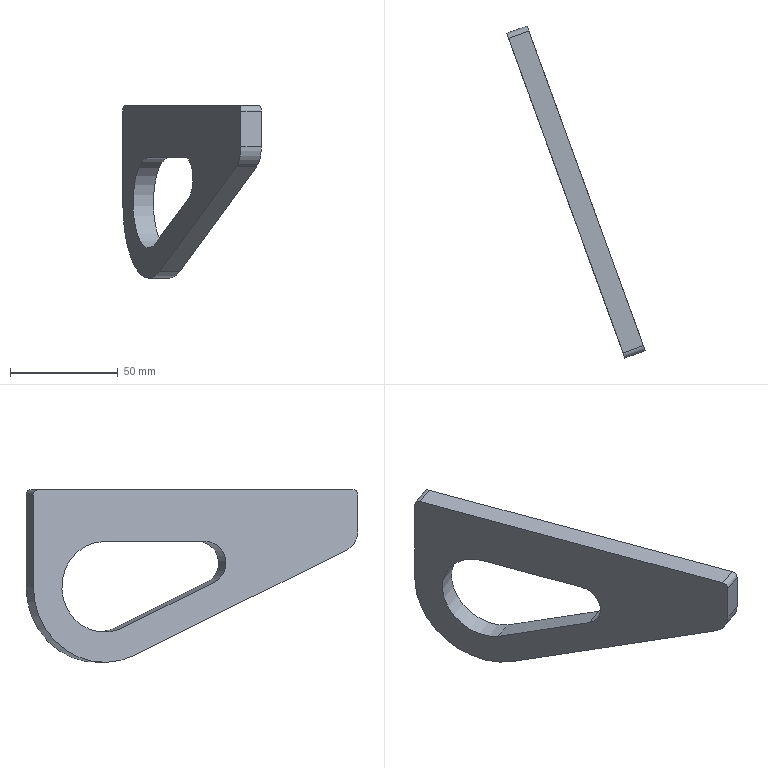Part | STEP file | Input 13 | 1 solid | 14 faces | box 64.12 x 153.771 x 80 mm | volume 68539 mm3 | plane 8 | cylinder 6 | commonest cylinder face diameters 5 x2 19.776 x1 20 x1 42 x1 70 x1
STEP:
#1=CARTESIAN_POINT('',(0.,0.,0.));
#2=DIRECTION('',(0.,0.,1.));
#3=DIRECTION('',(1.,0.,0.));
#4=AXIS2_PLACEMENT_3D('',#1,#2,#3);
#5=CARTESIAN_POINT('',(-156.648,51.655,-248.022));
#6=VERTEX_POINT('',#5);
#7=CARTESIAN_POINT('',(-154.674,46.229,-238.959));
#8=VERTEX_POINT('',#7);
#9=CARTESIAN_POINT('',(-158.094,55.626,-238.959));
#10=DIRECTION('',(-0.9397,-0.342,0.));
#11=DIRECTION('',(0.,0.,-1.));
#12=AXIS2_PLACEMENT_3D('',#9,#10,#11);
#13=CIRCLE('',#12,10.);
#14=CARTESIAN_POINT('',(-148.697,59.046,-238.959));
#15=DIRECTION('',(-0.9397,-0.342,0.));
#16=DIRECTION('',(0.,0.,1.));
#17=AXIS2_PLACEMENT_3D('',#14,#15,#16);
#18=CYLINDRICAL_SURFACE('',#17,10.);
#19=CARTESIAN_POINT('',(3.142,10.));
#20=DIRECTION('',(1.,0.));
#21=VECTOR('',#20,1.);
#22=LINE('',#19,#21);
#23=(GEOMETRIC_REPRESENTATION_CONTEXT(2)PARAMETRIC_REPRESENTATION_CONTEXT()REPRESENTATION_CONTEXT('',''));
#24=DEFINITIONAL_REPRESENTATION('',(#22),#23);
#25=PCURVE('',#18,#24);
#26=CARTESIAN_POINT('',(-158.094,55.626,-238.959));
#27=DIRECTION('',(0.9397,0.342,0.));
#28=DIRECTION('',(0.,0.,-1.));
#29=AXIS2_PLACEMENT_3D('',#26,#27,#28);
#30=PLANE('',#29);
#31=CARTESIAN_POINT('',(10.,0.));
#32=CARTESIAN_POINT('',(10.,-17.321));
#33=CARTESIAN_POINT('',(-5.,-8.66));
#34=CARTESIAN_POINT('',(-20.,0.));
#35=CARTESIAN_POINT('',(-5.,8.66));
#36=CARTESIAN_POINT('',(10.,17.321));
#37=CARTESIAN_POINT('',(10.,0.));
#38=(BOUNDED_CURVE()B_SPLINE_CURVE(2,(#31,#32,#33,#34,#35,#36,#37),.UNSPECIFIED.,.T.,.F.)B_SPLINE_CURVE_WITH_KNOTS((1,2,2,2,2,1),(-2.094,0.,2.094,4.189,6.283,8.378),.UNSPECIFIED.)CURVE()GEOMETRIC_REPRESENTATION_ITEM()RATIONAL_B_SPLINE_CURVE((1.,0.5,1.,0.5,1.,0.5,1.))REPRESENTATION_ITEM(''));
#39=(GEOMETRIC_REPRESENTATION_CONTEXT(2)PARAMETRIC_REPRESENTATION_CONTEXT()REPRESENTATION_CONTEXT('',''));
#40=DEFINITIONAL_REPRESENTATION('',(#38),#39);
#41=PCURVE('',#30,#40);
#42=SURFACE_CURVE('',#13,(#25,#41),.PCURVE_S1.);
#43=EDGE_CURVE('',#6,#8,#42,.T.);
#44=ORIENTED_EDGE('',*,*,#43,.F.);
#45=CARTESIAN_POINT('',(-147.252,55.075,-248.022));
#46=VERTEX_POINT('',#45);
#47=CARTESIAN_POINT('',(-147.252,55.075,-248.022));
#48=DIRECTION('',(-0.9397,-0.342,0.));
#49=VECTOR('',#48,1.);
#50=LINE('',#47,#49);
#51=CARTESIAN_POINT('',(3.578,0.));
#52=DIRECTION('',(0.,1.));
#53=VECTOR('',#52,1.);
#54=LINE('',#51,#53);
#55=(GEOMETRIC_REPRESENTATION_CONTEXT(2)PARAMETRIC_REPRESENTATION_CONTEXT()REPRESENTATION_CONTEXT('',''));
#56=DEFINITIONAL_REPRESENTATION('',(#54),#55);
#57=PCURVE('',#18,#56);
#58=CARTESIAN_POINT('',(-147.252,55.075,-248.022));
#59=DIRECTION('',(0.1445,-0.3971,-0.9063));
#60=DIRECTION('',(0.31,-0.8517,0.4226));
#61=AXIS2_PLACEMENT_3D('',#58,#59,#60);
#62=PLANE('',#61);
#63=CARTESIAN_POINT('',(0.,0.));
#64=DIRECTION('',(0.,1.));
#65=VECTOR('',#64,1.);
#66=LINE('',#63,#65);
#67=(GEOMETRIC_REPRESENTATION_CONTEXT(2)PARAMETRIC_REPRESENTATION_CONTEXT()REPRESENTATION_CONTEXT('',''));
#68=DEFINITIONAL_REPRESENTATION('',(#66),#67);
#69=PCURVE('',#62,#68);
#70=SURFACE_CURVE('',#50,(#57,#69),.PCURVE_S1.);
#71=EDGE_CURVE('',#46,#6,#70,.T.);
#72=ORIENTED_EDGE('',*,*,#71,.F.);
#73=CARTESIAN_POINT('',(-145.277,49.649,-238.959));
#74=VERTEX_POINT('',#73);
#75=CARTESIAN_POINT('',(-148.697,59.046,-238.959));
#76=DIRECTION('',(-0.9397,-0.342,0.));
#77=DIRECTION('',(0.,0.,-1.));
#78=AXIS2_PLACEMENT_3D('',#75,#76,#77);
#79=CIRCLE('',#78,10.);
#80=CARTESIAN_POINT('',(3.142,0.));
#81=DIRECTION('',(1.,0.));
#82=VECTOR('',#81,1.);
#83=LINE('',#80,#82);
#84=(GEOMETRIC_REPRESENTATION_CONTEXT(2)PARAMETRIC_REPRESENTATION_CONTEXT()REPRESENTATION_CONTEXT('',''));
#85=DEFINITIONAL_REPRESENTATION('',(#83),#84);
#86=PCURVE('',#18,#85);
#87=CARTESIAN_POINT('',(-148.697,59.046,-238.959));
#88=DIRECTION('',(0.9397,0.342,0.));
#89=DIRECTION('',(0.,0.,-1.));
#90=AXIS2_PLACEMENT_3D('',#87,#88,#89);
#91=PLANE('',#90);
#92=CARTESIAN_POINT('',(10.,0.));
#93=CARTESIAN_POINT('',(10.,-17.321));
#94=CARTESIAN_POINT('',(-5.,-8.66));
#95=CARTESIAN_POINT('',(-20.,0.));
#96=CARTESIAN_POINT('',(-5.,8.66));
#97=CARTESIAN_POINT('',(10.,17.321));
#98=CARTESIAN_POINT('',(10.,0.));
#99=(BOUNDED_CURVE()B_SPLINE_CURVE(2,(#92,#93,#94,#95,#96,#97,#98),.UNSPECIFIED.,.T.,.F.)B_SPLINE_CURVE_WITH_KNOTS((1,2,2,2,2,1),(-2.094,0.,2.094,4.189,6.283,8.378),.UNSPECIFIED.)CURVE()GEOMETRIC_REPRESENTATION_ITEM()RATIONAL_B_SPLINE_CURVE((1.,0.5,1.,0.5,1.,0.5,1.))REPRESENTATION_ITEM(''));
#100=(GEOMETRIC_REPRESENTATION_CONTEXT(2)PARAMETRIC_REPRESENTATION_CONTEXT()REPRESENTATION_CONTEXT('',''));
#101=DEFINITIONAL_REPRESENTATION('',(#99),#100);
#102=PCURVE('',#91,#101);
#103=SURFACE_CURVE('',#79,(#86,#102),.PCURVE_S1.);
#104=EDGE_CURVE('',#46,#74,#103,.T.);
#105=ORIENTED_EDGE('',*,*,#104,.T.);
#106=CARTESIAN_POINT('',(-145.277,49.649,-238.959));
#107=DIRECTION('',(-0.9397,-0.342,0.));
#108=VECTOR('',#107,1.);
#109=LINE('',#106,#108);
#110=CARTESIAN_POINT('',(4.712,0.));
#111=DIRECTION('',(0.,1.));
#112=VECTOR('',#111,1.);
#113=LINE('',#110,#112);
#114=(GEOMETRIC_REPRESENTATION_CONTEXT(2)PARAMETRIC_REPRESENTATION_CONTEXT()REPRESENTATION_CONTEXT('',''));
#115=DEFINITIONAL_REPRESENTATION('',(#113),#114);
#116=PCURVE('',#18,#115);
#117=CARTESIAN_POINT('',(-145.277,49.649,-222.5));
#118=DIRECTION('',(0.342,-0.9397,0.));
#119=DIRECTION('',(0.9397,0.342,0.));
#120=AXIS2_PLACEMENT_3D('',#117,#118,#119);
#121=PLANE('',#120);
#122=CARTESIAN_POINT('',(0.,-16.459));
#123=DIRECTION('',(-1.,0.));
#124=VECTOR('',#123,1.);
#125=LINE('',#122,#124);
#126=(GEOMETRIC_REPRESENTATION_CONTEXT(2)PARAMETRIC_REPRESENTATION_CONTEXT()REPRESENTATION_CONTEXT('',''));
#127=DEFINITIONAL_REPRESENTATION('',(#125),#126);
#128=PCURVE('',#121,#127);
#129=SURFACE_CURVE('',#109,(#116,#128),.PCURVE_S1.);
#130=EDGE_CURVE('',#74,#8,#129,.T.);
#131=ORIENTED_EDGE('',*,*,#130,.T.);
#132=EDGE_LOOP('',(#44,#72,#105,#131));
#133=FACE_BOUND('',#132,.T.);
#134=ADVANCED_FACE('',(#133),#18,.T.);
#135=CARTESIAN_POINT('',(-192.367,149.791,-296.721));
#136=VERTEX_POINT('',#135);
#137=CARTESIAN_POINT('',(-156.648,51.655,-248.022));
#138=DIRECTION('',(0.31,-0.8517,0.4226));
#139=VECTOR('',#138,1.);
#140=LINE('',#137,#139);
#141=CARTESIAN_POINT('',(0.,10.));
#142=DIRECTION('',(1.,0.));
#143=VECTOR('',#142,1.);
#144=LINE('',#141,#143);
#145=(GEOMETRIC_REPRESENTATION_CONTEXT(2)PARAMETRIC_REPRESENTATION_CONTEXT()REPRESENTATION_CONTEXT('',''));
#146=DEFINITIONAL_REPRESENTATION('',(#144),#145);
#147=PCURVE('',#62,#146);
#148=CARTESIAN_POINT('',(9.063,-4.226));
#149=DIRECTION('',(-0.4226,-0.9063));
#150=VECTOR('',#149,1.);
#151=LINE('',#148,#150);
#152=(GEOMETRIC_REPRESENTATION_CONTEXT(2)PARAMETRIC_REPRESENTATION_CONTEXT()REPRESENTATION_CONTEXT('',''));
#153=DEFINITIONAL_REPRESENTATION('',(#151),#152);
#154=PCURVE('',#30,#153);
#155=SURFACE_CURVE('',#140,(#147,#154),.PCURVE_S1.);
#156=EDGE_CURVE('',#136,#6,#155,.T.);
#157=ORIENTED_EDGE('',*,*,#156,.F.);
#158=CARTESIAN_POINT('',(-182.97,153.211,-296.721));
#159=VERTEX_POINT('',#158);
#160=CARTESIAN_POINT('',(-182.97,153.211,-296.721));
#161=DIRECTION('',(-0.9397,-0.342,0.));
#162=VECTOR('',#161,1.);
#163=LINE('',#160,#162);
#164=CARTESIAN_POINT('',(-115.231,0.));
#165=DIRECTION('',(0.,1.));
#166=VECTOR('',#165,1.);
#167=LINE('',#164,#166);
#168=(GEOMETRIC_REPRESENTATION_CONTEXT(2)PARAMETRIC_REPRESENTATION_CONTEXT()REPRESENTATION_CONTEXT('',''));
#169=DEFINITIONAL_REPRESENTATION('',(#167),#168);
#170=PCURVE('',#62,#169);
#171=CARTESIAN_POINT('',(-188.029,167.111,-265.));
#172=DIRECTION('',(-0.9397,-0.342,0.));
#173=DIRECTION('',(0.,0.,1.));
#174=AXIS2_PLACEMENT_3D('',#171,#172,#173);
#175=CYLINDRICAL_SURFACE('',#174,35.);
#176=CARTESIAN_POINT('',(3.578,0.));
#177=DIRECTION('',(0.,1.));
#178=VECTOR('',#177,1.);
#179=LINE('',#176,#178);
#180=(GEOMETRIC_REPRESENTATION_CONTEXT(2)PARAMETRIC_REPRESENTATION_CONTEXT()REPRESENTATION_CONTEXT('',''));
#181=DEFINITIONAL_REPRESENTATION('',(#179),#180);
#182=PCURVE('',#175,#181);
#183=SURFACE_CURVE('',#163,(#170,#182),.PCURVE_S1.);
#184=EDGE_CURVE('',#159,#136,#183,.T.);
#185=ORIENTED_EDGE('',*,*,#184,.F.);
#186=CARTESIAN_POINT('',(-147.252,55.075,-248.022));
#187=DIRECTION('',(0.31,-0.8517,0.4226));
#188=VECTOR('',#187,1.);
#189=LINE('',#186,#188);
#190=CARTESIAN_POINT('',(0.,0.));
#191=DIRECTION('',(1.,0.));
#192=VECTOR('',#191,1.);
#193=LINE('',#190,#192);
#194=(GEOMETRIC_REPRESENTATION_CONTEXT(2)PARAMETRIC_REPRESENTATION_CONTEXT()REPRESENTATION_CONTEXT('',''));
#195=DEFINITIONAL_REPRESENTATION('',(#193),#194);
#196=PCURVE('',#62,#195);
#197=CARTESIAN_POINT('',(9.063,-4.226));
#198=DIRECTION('',(-0.4226,-0.9063));
#199=VECTOR('',#198,1.);
#200=LINE('',#197,#199);
#201=(GEOMETRIC_REPRESENTATION_CONTEXT(2)PARAMETRIC_REPRESENTATION_CONTEXT()REPRESENTATION_CONTEXT('',''));
#202=DEFINITIONAL_REPRESENTATION('',(#200),#201);
#203=PCURVE('',#91,#202);
#204=SURFACE_CURVE('',#189,(#196,#203),.PCURVE_S1.);
#205=EDGE_CURVE('',#159,#46,#204,.T.);
#206=ORIENTED_EDGE('',*,*,#205,.T.);
#207=ORIENTED_EDGE('',*,*,#71,.T.);
#208=EDGE_LOOP('',(#157,#185,#206,#207));
#209=FACE_BOUND('',#208,.T.);
#210=ADVANCED_FACE('',(#209),#62,.T.);
#211=CARTESIAN_POINT('',(-209.397,196.58,-265.));
#212=VERTEX_POINT('',#211);
#213=CARTESIAN_POINT('',(-197.426,163.691,-265.));
#214=DIRECTION('',(-0.9397,-0.342,0.));
#215=DIRECTION('',(0.,0.,1.));
#216=AXIS2_PLACEMENT_3D('',#213,#214,#215);
#217=CIRCLE('',#216,35.);
#218=CARTESIAN_POINT('',(0.,10.));
#219=DIRECTION('',(1.,0.));
#220=VECTOR('',#219,1.);
#221=LINE('',#218,#220);
#222=(GEOMETRIC_REPRESENTATION_CONTEXT(2)PARAMETRIC_REPRESENTATION_CONTEXT()REPRESENTATION_CONTEXT('',''));
#223=DEFINITIONAL_REPRESENTATION('',(#221),#222);
#224=PCURVE('',#175,#223);
#225=CARTESIAN_POINT('',(-8.959,115.));
#226=CARTESIAN_POINT('',(-8.959,175.622));
#227=CARTESIAN_POINT('',(43.541,145.311));
#228=CARTESIAN_POINT('',(96.041,115.));
#229=CARTESIAN_POINT('',(43.541,84.689));
#230=CARTESIAN_POINT('',(-8.959,54.378));
#231=CARTESIAN_POINT('',(-8.959,115.));
#232=(BOUNDED_CURVE()B_SPLINE_CURVE(2,(#225,#226,#227,#228,#229,#230,#231),.UNSPECIFIED.,.T.,.F.)B_SPLINE_CURVE_WITH_KNOTS((1,2,2,2,2,1),(-2.094,0.,2.094,4.189,6.283,8.378),.UNSPECIFIED.)CURVE()GEOMETRIC_REPRESENTATION_ITEM()RATIONAL_B_SPLINE_CURVE((1.,0.5,1.,0.5,1.,0.5,1.))REPRESENTATION_ITEM(''));
#233=(GEOMETRIC_REPRESENTATION_CONTEXT(2)PARAMETRIC_REPRESENTATION_CONTEXT()REPRESENTATION_CONTEXT('',''));
#234=DEFINITIONAL_REPRESENTATION('',(#232),#233);
#235=PCURVE('',#30,#234);
#236=SURFACE_CURVE('',#217,(#224,#235),.PCURVE_S1.);
#237=EDGE_CURVE('',#212,#136,#236,.T.);
#238=ORIENTED_EDGE('',*,*,#237,.F.);
#239=CARTESIAN_POINT('',(-200.,200.,-265.));
#240=VERTEX_POINT('',#239);
#241=CARTESIAN_POINT('',(-200.,200.,-265.));
#242=DIRECTION('',(-0.9397,-0.342,0.));
#243=VECTOR('',#242,1.);
#244=LINE('',#241,#243);
#245=CARTESIAN_POINT('',(1.571,0.));
#246=DIRECTION('',(0.,1.));
#247=VECTOR('',#246,1.);
#248=LINE('',#245,#247);
#249=(GEOMETRIC_REPRESENTATION_CONTEXT(2)PARAMETRIC_REPRESENTATION_CONTEXT()REPRESENTATION_CONTEXT('',''));
#250=DEFINITIONAL_REPRESENTATION('',(#248),#249);
#251=PCURVE('',#175,#250);
#252=CARTESIAN_POINT('',(-200.,200.,-222.5));
#253=DIRECTION('',(-0.342,0.9397,0.));
#254=DIRECTION('',(0.,0.,-1.));
#255=AXIS2_PLACEMENT_3D('',#252,#253,#254);
#256=PLANE('',#255);
#257=CARTESIAN_POINT('',(42.5,0.));
#258=DIRECTION('',(0.,1.));
#259=VECTOR('',#258,1.);
#260=LINE('',#257,#259);
#261=(GEOMETRIC_REPRESENTATION_CONTEXT(2)PARAMETRIC_REPRESENTATION_CONTEXT()REPRESENTATION_CONTEXT('',''));
#262=DEFINITIONAL_REPRESENTATION('',(#260),#261);
#263=PCURVE('',#256,#262);
#264=SURFACE_CURVE('',#244,(#251,#263),.PCURVE_S1.);
#265=EDGE_CURVE('',#240,#212,#264,.T.);
#266=ORIENTED_EDGE('',*,*,#265,.F.);
#267=CARTESIAN_POINT('',(-188.029,167.111,-265.));
#268=DIRECTION('',(-0.9397,-0.342,0.));
#269=DIRECTION('',(0.,0.,1.));
#270=AXIS2_PLACEMENT_3D('',#267,#268,#269);
#271=CIRCLE('',#270,35.);
#272=CARTESIAN_POINT('',(0.,0.));
#273=DIRECTION('',(1.,0.));
#274=VECTOR('',#273,1.);
#275=LINE('',#272,#274);
#276=(GEOMETRIC_REPRESENTATION_CONTEXT(2)PARAMETRIC_REPRESENTATION_CONTEXT()REPRESENTATION_CONTEXT('',''));
#277=DEFINITIONAL_REPRESENTATION('',(#275),#276);
#278=PCURVE('',#175,#277);
#279=CARTESIAN_POINT('',(-8.959,115.));
#280=CARTESIAN_POINT('',(-8.959,175.622));
#281=CARTESIAN_POINT('',(43.541,145.311));
#282=CARTESIAN_POINT('',(96.041,115.));
#283=CARTESIAN_POINT('',(43.541,84.689));
#284=CARTESIAN_POINT('',(-8.959,54.378));
#285=CARTESIAN_POINT('',(-8.959,115.));
#286=(BOUNDED_CURVE()B_SPLINE_CURVE(2,(#279,#280,#281,#282,#283,#284,#285),.UNSPECIFIED.,.T.,.F.)B_SPLINE_CURVE_WITH_KNOTS((1,2,2,2,2,1),(-2.094,0.,2.094,4.189,6.283,8.378),.UNSPECIFIED.)CURVE()GEOMETRIC_REPRESENTATION_ITEM()RATIONAL_B_SPLINE_CURVE((1.,0.5,1.,0.5,1.,0.5,1.))REPRESENTATION_ITEM(''));
#287=(GEOMETRIC_REPRESENTATION_CONTEXT(2)PARAMETRIC_REPRESENTATION_CONTEXT()REPRESENTATION_CONTEXT('',''));
#288=DEFINITIONAL_REPRESENTATION('',(#286),#287);
#289=PCURVE('',#91,#288);
#290=SURFACE_CURVE('',#271,(#278,#289),.PCURVE_S1.);
#291=EDGE_CURVE('',#240,#159,#290,.T.);
#292=ORIENTED_EDGE('',*,*,#291,.T.);
#293=ORIENTED_EDGE('',*,*,#184,.T.);
#294=EDGE_LOOP('',(#238,#266,#292,#293));
#295=FACE_BOUND('',#294,.T.);
#296=ADVANCED_FACE('',(#295),#175,.T.);
#297=CARTESIAN_POINT('',(-209.397,196.58,-222.5));
#298=VERTEX_POINT('',#297);
#299=CARTESIAN_POINT('',(-209.397,196.58,-222.5));
#300=DIRECTION('',(0.,0.,-1.));
#301=VECTOR('',#300,1.);
#302=LINE('',#299,#301);
#303=CARTESIAN_POINT('',(0.,10.));
#304=DIRECTION('',(1.,0.));
#305=VECTOR('',#304,1.);
#306=LINE('',#303,#305);
#307=(GEOMETRIC_REPRESENTATION_CONTEXT(2)PARAMETRIC_REPRESENTATION_CONTEXT()REPRESENTATION_CONTEXT('',''));
#308=DEFINITIONAL_REPRESENTATION('',(#306),#307);
#309=PCURVE('',#256,#308);
#310=CARTESIAN_POINT('',(-16.459,150.));
#311=DIRECTION('',(1.,0.));
#312=VECTOR('',#311,1.);
#313=LINE('',#310,#312);
#314=(GEOMETRIC_REPRESENTATION_CONTEXT(2)PARAMETRIC_REPRESENTATION_CONTEXT()REPRESENTATION_CONTEXT('',''));
#315=DEFINITIONAL_REPRESENTATION('',(#313),#314);
#316=PCURVE('',#30,#315);
#317=SURFACE_CURVE('',#302,(#309,#316),.PCURVE_S1.);
#318=EDGE_CURVE('',#298,#212,#317,.T.);
#319=ORIENTED_EDGE('',*,*,#318,.F.);
#320=CARTESIAN_POINT('',(-200.,200.,-222.5));
#321=VERTEX_POINT('',#320);
#322=CARTESIAN_POINT('',(-200.,200.,-222.5));
#323=DIRECTION('',(-0.9397,-0.342,0.));
#324=VECTOR('',#323,1.);
#325=LINE('',#322,#324);
#326=CARTESIAN_POINT('',(0.,0.));
#327=DIRECTION('',(0.,1.));
#328=VECTOR('',#327,1.);
#329=LINE('',#326,#328);
#330=(GEOMETRIC_REPRESENTATION_CONTEXT(2)PARAMETRIC_REPRESENTATION_CONTEXT()REPRESENTATION_CONTEXT('',''));
#331=DEFINITIONAL_REPRESENTATION('',(#329),#330);
#332=PCURVE('',#256,#331);
#333=CARTESIAN_POINT('',(-199.145,197.651,-222.5));
#334=DIRECTION('',(-0.9397,-0.342,0.));
#335=DIRECTION('',(0.,0.,1.));
#336=AXIS2_PLACEMENT_3D('',#333,#334,#335);
#337=CYLINDRICAL_SURFACE('',#336,2.5);
#338=CARTESIAN_POINT('',(1.571,0.));
#339=DIRECTION('',(0.,1.));
#340=VECTOR('',#339,1.);
#341=LINE('',#338,#340);
#342=(GEOMETRIC_REPRESENTATION_CONTEXT(2)PARAMETRIC_REPRESENTATION_CONTEXT()REPRESENTATION_CONTEXT('',''));
#343=DEFINITIONAL_REPRESENTATION('',(#341),#342);
#344=PCURVE('',#337,#343);
#345=SURFACE_CURVE('',#325,(#332,#344),.PCURVE_S1.);
#346=EDGE_CURVE('',#321,#298,#345,.T.);
#347=ORIENTED_EDGE('',*,*,#346,.F.);
#348=CARTESIAN_POINT('',(-200.,200.,-222.5));
#349=DIRECTION('',(0.,0.,-1.));
#350=VECTOR('',#349,1.);
#351=LINE('',#348,#350);
#352=CARTESIAN_POINT('',(0.,0.));
#353=DIRECTION('',(1.,0.));
#354=VECTOR('',#353,1.);
#355=LINE('',#352,#354);
#356=(GEOMETRIC_REPRESENTATION_CONTEXT(2)PARAMETRIC_REPRESENTATION_CONTEXT()REPRESENTATION_CONTEXT('',''));
#357=DEFINITIONAL_REPRESENTATION('',(#355),#356);
#358=PCURVE('',#256,#357);
#359=CARTESIAN_POINT('',(-16.459,150.));
#360=DIRECTION('',(1.,0.));
#361=VECTOR('',#360,1.);
#362=LINE('',#359,#361);
#363=(GEOMETRIC_REPRESENTATION_CONTEXT(2)PARAMETRIC_REPRESENTATION_CONTEXT()REPRESENTATION_CONTEXT('',''));
#364=DEFINITIONAL_REPRESENTATION('',(#362),#363);
#365=PCURVE('',#91,#364);
#366=SURFACE_CURVE('',#351,(#358,#365),.PCURVE_S1.);
#367=EDGE_CURVE('',#321,#240,#366,.T.);
#368=ORIENTED_EDGE('',*,*,#367,.T.);
#369=ORIENTED_EDGE('',*,*,#265,.T.);
#370=EDGE_LOOP('',(#319,#347,#368,#369));
#371=FACE_BOUND('',#370,.T.);
#372=ADVANCED_FACE('',(#371),#256,.T.);
#373=CARTESIAN_POINT('',(-208.542,194.231,-220.));
#374=VERTEX_POINT('',#373);
#375=CARTESIAN_POINT('',(-208.542,194.231,-222.5));
#376=DIRECTION('',(-0.9397,-0.342,0.));
#377=DIRECTION('',(0.,0.,1.));
#378=AXIS2_PLACEMENT_3D('',#375,#376,#377);
#379=CIRCLE('',#378,2.5);
#380=CARTESIAN_POINT('',(0.,10.));
#381=DIRECTION('',(1.,0.));
#382=VECTOR('',#381,1.);
#383=LINE('',#380,#382);
#384=(GEOMETRIC_REPRESENTATION_CONTEXT(2)PARAMETRIC_REPRESENTATION_CONTEXT()REPRESENTATION_CONTEXT('',''));
#385=DEFINITIONAL_REPRESENTATION('',(#383),#384);
#386=PCURVE('',#337,#385);
#387=CARTESIAN_POINT('',(-18.959,147.5));
#388=CARTESIAN_POINT('',(-18.959,151.83));
#389=CARTESIAN_POINT('',(-15.209,149.665));
#390=CARTESIAN_POINT('',(-11.459,147.5));
#391=CARTESIAN_POINT('',(-15.209,145.335));
#392=CARTESIAN_POINT('',(-18.959,143.17));
#393=CARTESIAN_POINT('',(-18.959,147.5));
#394=(BOUNDED_CURVE()B_SPLINE_CURVE(2,(#387,#388,#389,#390,#391,#392,#393),.UNSPECIFIED.,.T.,.F.)B_SPLINE_CURVE_WITH_KNOTS((1,2,2,2,2,1),(-2.094,0.,2.094,4.189,6.283,8.378),.UNSPECIFIED.)CURVE()GEOMETRIC_REPRESENTATION_ITEM()RATIONAL_B_SPLINE_CURVE((1.,0.5,1.,0.5,1.,0.5,1.))REPRESENTATION_ITEM(''));
#395=(GEOMETRIC_REPRESENTATION_CONTEXT(2)PARAMETRIC_REPRESENTATION_CONTEXT()REPRESENTATION_CONTEXT('',''));
#396=DEFINITIONAL_REPRESENTATION('',(#394),#395);
#397=PCURVE('',#30,#396);
#398=SURFACE_CURVE('',#379,(#386,#397),.PCURVE_S1.);
#399=EDGE_CURVE('',#374,#298,#398,.T.);
#400=ORIENTED_EDGE('',*,*,#399,.F.);
#401=CARTESIAN_POINT('',(-199.145,197.651,-220.));
#402=VERTEX_POINT('',#401);
#403=CARTESIAN_POINT('',(-199.145,197.651,-220.));
#404=DIRECTION('',(-0.9397,-0.342,0.));
#405=VECTOR('',#404,1.);
#406=LINE('',#403,#405);
#407=CARTESIAN_POINT('',(0.,0.));
#408=DIRECTION('',(0.,1.));
#409=VECTOR('',#408,1.);
#410=LINE('',#407,#409);
#411=(GEOMETRIC_REPRESENTATION_CONTEXT(2)PARAMETRIC_REPRESENTATION_CONTEXT()REPRESENTATION_CONTEXT('',''));
#412=DEFINITIONAL_REPRESENTATION('',(#410),#411);
#413=PCURVE('',#337,#412);
#414=CARTESIAN_POINT('',(-146.132,51.998,-220.));
#415=DIRECTION('',(0.,0.,1.));
#416=DIRECTION('',(-0.342,0.9397,0.));
#417=AXIS2_PLACEMENT_3D('',#414,#415,#416);
#418=PLANE('',#417);
#419=CARTESIAN_POINT('',(155.,0.));
#420=DIRECTION('',(0.,1.));
#421=VECTOR('',#420,1.);
#422=LINE('',#419,#421);
#423=(GEOMETRIC_REPRESENTATION_CONTEXT(2)PARAMETRIC_REPRESENTATION_CONTEXT()REPRESENTATION_CONTEXT('',''));
#424=DEFINITIONAL_REPRESENTATION('',(#422),#423);
#425=PCURVE('',#418,#424);
#426=SURFACE_CURVE('',#406,(#413,#425),.PCURVE_S1.);
#427=EDGE_CURVE('',#402,#374,#426,.T.);
#428=ORIENTED_EDGE('',*,*,#427,.F.);
#429=CARTESIAN_POINT('',(-199.145,197.651,-222.5));
#430=DIRECTION('',(-0.9397,-0.342,0.));
#431=DIRECTION('',(0.,0.,1.));
#432=AXIS2_PLACEMENT_3D('',#429,#430,#431);
#433=CIRCLE('',#432,2.5);
#434=CARTESIAN_POINT('',(0.,0.));
#435=DIRECTION('',(1.,0.));
#436=VECTOR('',#435,1.);
#437=LINE('',#434,#436);
#438=(GEOMETRIC_REPRESENTATION_CONTEXT(2)PARAMETRIC_REPRESENTATION_CONTEXT()REPRESENTATION_CONTEXT('',''));
#439=DEFINITIONAL_REPRESENTATION('',(#437),#438);
#440=PCURVE('',#337,#439);
#441=CARTESIAN_POINT('',(-18.959,147.5));
#442=CARTESIAN_POINT('',(-18.959,151.83));
#443=CARTESIAN_POINT('',(-15.209,149.665));
#444=CARTESIAN_POINT('',(-11.459,147.5));
#445=CARTESIAN_POINT('',(-15.209,145.335));
#446=CARTESIAN_POINT('',(-18.959,143.17));
#447=CARTESIAN_POINT('',(-18.959,147.5));
#448=(BOUNDED_CURVE()B_SPLINE_CURVE(2,(#441,#442,#443,#444,#445,#446,#447),.UNSPECIFIED.,.T.,.F.)B_SPLINE_CURVE_WITH_KNOTS((1,2,2,2,2,1),(-2.094,0.,2.094,4.189,6.283,8.378),.UNSPECIFIED.)CURVE()GEOMETRIC_REPRESENTATION_ITEM()RATIONAL_B_SPLINE_CURVE((1.,0.5,1.,0.5,1.,0.5,1.))REPRESENTATION_ITEM(''));
#449=(GEOMETRIC_REPRESENTATION_CONTEXT(2)PARAMETRIC_REPRESENTATION_CONTEXT()REPRESENTATION_CONTEXT('',''));
#450=DEFINITIONAL_REPRESENTATION('',(#448),#449);
#451=PCURVE('',#91,#450);
#452=SURFACE_CURVE('',#433,(#440,#451),.PCURVE_S1.);
#453=EDGE_CURVE('',#402,#321,#452,.T.);
#454=ORIENTED_EDGE('',*,*,#453,.T.);
#455=ORIENTED_EDGE('',*,*,#346,.T.);
#456=EDGE_LOOP('',(#400,#428,#454,#455));
#457=FACE_BOUND('',#456,.T.);
#458=ADVANCED_FACE('',(#457),#337,.T.);
#459=CARTESIAN_POINT('',(-155.529,48.578,-220.));
#460=VERTEX_POINT('',#459);
#461=CARTESIAN_POINT('',(-155.529,48.578,-220.));
#462=DIRECTION('',(-0.342,0.9397,0.));
#463=VECTOR('',#462,1.);
#464=LINE('',#461,#463);
#465=CARTESIAN_POINT('',(0.,10.));
#466=DIRECTION('',(1.,0.));
#467=VECTOR('',#466,1.);
#468=LINE('',#465,#467);
#469=(GEOMETRIC_REPRESENTATION_CONTEXT(2)PARAMETRIC_REPRESENTATION_CONTEXT()REPRESENTATION_CONTEXT('',''));
#470=DEFINITIONAL_REPRESENTATION('',(#468),#469);
#471=PCURVE('',#418,#470);
#472=CARTESIAN_POINT('',(-18.959,-7.5));
#473=DIRECTION('',(0.,1.));
#474=VECTOR('',#473,1.);
#475=LINE('',#472,#474);
#476=(GEOMETRIC_REPRESENTATION_CONTEXT(2)PARAMETRIC_REPRESENTATION_CONTEXT()REPRESENTATION_CONTEXT('',''));
#477=DEFINITIONAL_REPRESENTATION('',(#475),#476);
#478=PCURVE('',#30,#477);
#479=SURFACE_CURVE('',#464,(#471,#478),.PCURVE_S1.);
#480=EDGE_CURVE('',#460,#374,#479,.T.);
#481=ORIENTED_EDGE('',*,*,#480,.F.);
#482=CARTESIAN_POINT('',(-146.132,51.998,-220.));
#483=VERTEX_POINT('',#482);
#484=CARTESIAN_POINT('',(-146.132,51.998,-220.));
#485=DIRECTION('',(-0.9397,-0.342,0.));
#486=VECTOR('',#485,1.);
#487=LINE('',#484,#486);
#488=CARTESIAN_POINT('',(0.,0.));
#489=DIRECTION('',(0.,1.));
#490=VECTOR('',#489,1.);
#491=LINE('',#488,#490);
#492=(GEOMETRIC_REPRESENTATION_CONTEXT(2)PARAMETRIC_REPRESENTATION_CONTEXT()REPRESENTATION_CONTEXT('',''));
#493=DEFINITIONAL_REPRESENTATION('',(#491),#492);
#494=PCURVE('',#418,#493);
#495=CARTESIAN_POINT('',(-146.132,51.998,-222.5));
#496=DIRECTION('',(-0.9397,-0.342,0.));
#497=DIRECTION('',(0.,0.,1.));
#498=AXIS2_PLACEMENT_3D('',#495,#496,#497);
#499=CYLINDRICAL_SURFACE('',#498,2.5);
#500=CARTESIAN_POINT('',(6.283,0.));
#501=DIRECTION('',(0.,1.));
#502=VECTOR('',#501,1.);
#503=LINE('',#500,#502);
#504=(GEOMETRIC_REPRESENTATION_CONTEXT(2)PARAMETRIC_REPRESENTATION_CONTEXT()REPRESENTATION_CONTEXT('',''));
#505=DEFINITIONAL_REPRESENTATION('',(#503),#504);
#506=PCURVE('',#499,#505);
#507=SURFACE_CURVE('',#487,(#494,#506),.PCURVE_S1.);
#508=EDGE_CURVE('',#483,#460,#507,.T.);
#509=ORIENTED_EDGE('',*,*,#508,.F.);
#510=CARTESIAN_POINT('',(-146.132,51.998,-220.));
#511=DIRECTION('',(-0.342,0.9397,0.));
#512=VECTOR('',#511,1.);
#513=LINE('',#510,#512);
#514=CARTESIAN_POINT('',(0.,0.));
#515=DIRECTION('',(1.,0.));
#516=VECTOR('',#515,1.);
#517=LINE('',#514,#516);
#518=(GEOMETRIC_REPRESENTATION_CONTEXT(2)PARAMETRIC_REPRESENTATION_CONTEXT()REPRESENTATION_CONTEXT('',''));
#519=DEFINITIONAL_REPRESENTATION('',(#517),#518);
#520=PCURVE('',#418,#519);
#521=CARTESIAN_POINT('',(-18.959,-7.5));
#522=DIRECTION('',(0.,1.));
#523=VECTOR('',#522,1.);
#524=LINE('',#521,#523);
#525=(GEOMETRIC_REPRESENTATION_CONTEXT(2)PARAMETRIC_REPRESENTATION_CONTEXT()REPRESENTATION_CONTEXT('',''));
#526=DEFINITIONAL_REPRESENTATION('',(#524),#525);
#527=PCURVE('',#91,#526);
#528=SURFACE_CURVE('',#513,(#520,#527),.PCURVE_S1.);
#529=EDGE_CURVE('',#483,#402,#528,.T.);
#530=ORIENTED_EDGE('',*,*,#529,.T.);
#531=ORIENTED_EDGE('',*,*,#427,.T.);
#532=EDGE_LOOP('',(#481,#509,#530,#531));
#533=FACE_BOUND('',#532,.T.);
#534=ADVANCED_FACE('',(#533),#418,.T.);
#535=CARTESIAN_POINT('',(-154.674,46.229,-222.5));
#536=VERTEX_POINT('',#535);
#537=CARTESIAN_POINT('',(-155.529,48.578,-222.5));
#538=DIRECTION('',(-0.9397,-0.342,0.));
#539=DIRECTION('',(0.,0.,-1.));
#540=AXIS2_PLACEMENT_3D('',#537,#538,#539);
#541=CIRCLE('',#540,2.5);
#542=CARTESIAN_POINT('',(3.142,10.));
#543=DIRECTION('',(1.,0.));
#544=VECTOR('',#543,1.);
#545=LINE('',#542,#544);
#546=(GEOMETRIC_REPRESENTATION_CONTEXT(2)PARAMETRIC_REPRESENTATION_CONTEXT()REPRESENTATION_CONTEXT('',''));
#547=DEFINITIONAL_REPRESENTATION('',(#545),#546);
#548=PCURVE('',#499,#547);
#549=CARTESIAN_POINT('',(-13.959,-7.5));
#550=CARTESIAN_POINT('',(-13.959,-11.83));
#551=CARTESIAN_POINT('',(-17.709,-9.665));
#552=CARTESIAN_POINT('',(-21.459,-7.5));
#553=CARTESIAN_POINT('',(-17.709,-5.335));
#554=CARTESIAN_POINT('',(-13.959,-3.17));
#555=CARTESIAN_POINT('',(-13.959,-7.5));
#556=(BOUNDED_CURVE()B_SPLINE_CURVE(2,(#549,#550,#551,#552,#553,#554,#555),.UNSPECIFIED.,.T.,.F.)B_SPLINE_CURVE_WITH_KNOTS((1,2,2,2,2,1),(-2.094,0.,2.094,4.189,6.283,8.378),.UNSPECIFIED.)CURVE()GEOMETRIC_REPRESENTATION_ITEM()RATIONAL_B_SPLINE_CURVE((1.,0.5,1.,0.5,1.,0.5,1.))REPRESENTATION_ITEM(''));
#557=(GEOMETRIC_REPRESENTATION_CONTEXT(2)PARAMETRIC_REPRESENTATION_CONTEXT()REPRESENTATION_CONTEXT('',''));
#558=DEFINITIONAL_REPRESENTATION('',(#556),#557);
#559=PCURVE('',#30,#558);
#560=SURFACE_CURVE('',#541,(#548,#559),.PCURVE_S1.);
#561=EDGE_CURVE('',#536,#460,#560,.T.);
#562=ORIENTED_EDGE('',*,*,#561,.F.);
#563=CARTESIAN_POINT('',(-145.277,49.649,-222.5));
#564=VERTEX_POINT('',#563);
#565=CARTESIAN_POINT('',(-145.277,49.649,-222.5));
#566=DIRECTION('',(-0.9397,-0.342,0.));
#567=VECTOR('',#566,1.);
#568=LINE('',#565,#567);
#569=CARTESIAN_POINT('',(4.712,0.));
#570=DIRECTION('',(0.,1.));
#571=VECTOR('',#570,1.);
#572=LINE('',#569,#571);
#573=(GEOMETRIC_REPRESENTATION_CONTEXT(2)PARAMETRIC_REPRESENTATION_CONTEXT()REPRESENTATION_CONTEXT('',''));
#574=DEFINITIONAL_REPRESENTATION('',(#572),#573);
#575=PCURVE('',#499,#574);
#576=CARTESIAN_POINT('',(0.,0.));
#577=DIRECTION('',(-1.,0.));
#578=VECTOR('',#577,1.);
#579=LINE('',#576,#578);
#580=(GEOMETRIC_REPRESENTATION_CONTEXT(2)PARAMETRIC_REPRESENTATION_CONTEXT()REPRESENTATION_CONTEXT('',''));
#581=DEFINITIONAL_REPRESENTATION('',(#579),#580);
#582=PCURVE('',#121,#581);
#583=SURFACE_CURVE('',#568,(#575,#582),.PCURVE_S1.);
#584=EDGE_CURVE('',#564,#536,#583,.T.);
#585=ORIENTED_EDGE('',*,*,#584,.F.);
#586=CARTESIAN_POINT('',(-146.132,51.998,-222.5));
#587=DIRECTION('',(-0.9397,-0.342,0.));
#588=DIRECTION('',(0.,0.,-1.));
#589=AXIS2_PLACEMENT_3D('',#586,#587,#588);
#590=CIRCLE('',#589,2.5);
#591=CARTESIAN_POINT('',(3.142,0.));
#592=DIRECTION('',(1.,0.));
#593=VECTOR('',#592,1.);
#594=LINE('',#591,#593);
#595=(GEOMETRIC_REPRESENTATION_CONTEXT(2)PARAMETRIC_REPRESENTATION_CONTEXT()REPRESENTATION_CONTEXT('',''));
#596=DEFINITIONAL_REPRESENTATION('',(#594),#595);
#597=PCURVE('',#499,#596);
#598=CARTESIAN_POINT('',(-13.959,-7.5));
#599=CARTESIAN_POINT('',(-13.959,-11.83));
#600=CARTESIAN_POINT('',(-17.709,-9.665));
#601=CARTESIAN_POINT('',(-21.459,-7.5));
#602=CARTESIAN_POINT('',(-17.709,-5.335));
#603=CARTESIAN_POINT('',(-13.959,-3.17));
#604=CARTESIAN_POINT('',(-13.959,-7.5));
#605=(BOUNDED_CURVE()B_SPLINE_CURVE(2,(#598,#599,#600,#601,#602,#603,#604),.UNSPECIFIED.,.T.,.F.)B_SPLINE_CURVE_WITH_KNOTS((1,2,2,2,2,1),(-2.094,0.,2.094,4.189,6.283,8.378),.UNSPECIFIED.)CURVE()GEOMETRIC_REPRESENTATION_ITEM()RATIONAL_B_SPLINE_CURVE((1.,0.5,1.,0.5,1.,0.5,1.))REPRESENTATION_ITEM(''));
#606=(GEOMETRIC_REPRESENTATION_CONTEXT(2)PARAMETRIC_REPRESENTATION_CONTEXT()REPRESENTATION_CONTEXT('',''));
#607=DEFINITIONAL_REPRESENTATION('',(#605),#606);
#608=PCURVE('',#91,#607);
#609=SURFACE_CURVE('',#590,(#597,#608),.PCURVE_S1.);
#610=EDGE_CURVE('',#564,#483,#609,.T.);
#611=ORIENTED_EDGE('',*,*,#610,.T.);
#612=ORIENTED_EDGE('',*,*,#508,.T.);
#613=EDGE_LOOP('',(#562,#585,#611,#612));
#614=FACE_BOUND('',#613,.T.);
#615=ADVANCED_FACE('',(#614),#499,.T.);
#616=CARTESIAN_POINT('',(-154.674,46.229,-222.5));
#617=DIRECTION('',(0.,0.,1.));
#618=VECTOR('',#617,1.);
#619=LINE('',#616,#618);
#620=CARTESIAN_POINT('',(-10.,0.));
#621=DIRECTION('',(0.,1.));
#622=VECTOR('',#621,1.);
#623=LINE('',#620,#622);
#624=(GEOMETRIC_REPRESENTATION_CONTEXT(2)PARAMETRIC_REPRESENTATION_CONTEXT()REPRESENTATION_CONTEXT('',''));
#625=DEFINITIONAL_REPRESENTATION('',(#623),#624);
#626=PCURVE('',#121,#625);
#627=CARTESIAN_POINT('',(-16.459,-10.));
#628=DIRECTION('',(-1.,0.));
#629=VECTOR('',#628,1.);
#630=LINE('',#627,#629);
#631=(GEOMETRIC_REPRESENTATION_CONTEXT(2)PARAMETRIC_REPRESENTATION_CONTEXT()REPRESENTATION_CONTEXT('',''));
#632=DEFINITIONAL_REPRESENTATION('',(#630),#631);
#633=PCURVE('',#30,#632);
#634=SURFACE_CURVE('',#619,(#626,#633),.PCURVE_S1.);
#635=EDGE_CURVE('',#8,#536,#634,.T.);
#636=ORIENTED_EDGE('',*,*,#635,.F.);
#637=ORIENTED_EDGE('',*,*,#130,.F.);
#638=CARTESIAN_POINT('',(-145.277,49.649,-222.5));
#639=DIRECTION('',(0.,0.,1.));
#640=VECTOR('',#639,1.);
#641=LINE('',#638,#640);
#642=CARTESIAN_POINT('',(0.,0.));
#643=DIRECTION('',(0.,1.));
#644=VECTOR('',#643,1.);
#645=LINE('',#642,#644);
#646=(GEOMETRIC_REPRESENTATION_CONTEXT(2)PARAMETRIC_REPRESENTATION_CONTEXT()REPRESENTATION_CONTEXT('',''));
#647=DEFINITIONAL_REPRESENTATION('',(#645),#646);
#648=PCURVE('',#121,#647);
#649=CARTESIAN_POINT('',(-16.459,-10.));
#650=DIRECTION('',(-1.,0.));
#651=VECTOR('',#650,1.);
#652=LINE('',#649,#651);
#653=(GEOMETRIC_REPRESENTATION_CONTEXT(2)PARAMETRIC_REPRESENTATION_CONTEXT()REPRESENTATION_CONTEXT('',''));
#654=DEFINITIONAL_REPRESENTATION('',(#652),#653);
#655=PCURVE('',#91,#654);
#656=SURFACE_CURVE('',#641,(#648,#655),.PCURVE_S1.);
#657=EDGE_CURVE('',#74,#564,#656,.T.);
#658=ORIENTED_EDGE('',*,*,#657,.T.);
#659=ORIENTED_EDGE('',*,*,#584,.T.);
#660=EDGE_LOOP('',(#636,#637,#658,#659));
#661=FACE_BOUND('',#660,.T.);
#662=ADVANCED_FACE('',(#661),#121,.T.);
#663=CARTESIAN_POINT('',(-169.499,116.199,-262.85));
#664=VERTEX_POINT('',#663);
#665=CARTESIAN_POINT('',(-170.928,120.126,-244.));
#666=VERTEX_POINT('',#665);
#667=CARTESIAN_POINT('',(-170.928,120.126,-253.888));
#668=DIRECTION('',(-0.9397,-0.342,0.));
#669=DIRECTION('',(0.,0.,1.));
#670=AXIS2_PLACEMENT_3D('',#667,#668,#669);
#671=CIRCLE('',#670,9.888);
#672=CARTESIAN_POINT('',(5.041,65.));
#673=CARTESIAN_POINT('',(5.041,82.127));
#674=CARTESIAN_POINT('',(19.873,73.563));
#675=CARTESIAN_POINT('',(34.706,65.));
#676=CARTESIAN_POINT('',(19.873,56.437));
#677=CARTESIAN_POINT('',(5.041,47.873));
#678=CARTESIAN_POINT('',(5.041,65.));
#679=(BOUNDED_CURVE()B_SPLINE_CURVE(2,(#672,#673,#674,#675,#676,#677,#678),.UNSPECIFIED.,.T.,.F.)B_SPLINE_CURVE_WITH_KNOTS((1,2,2,2,2,1),(-2.094,0.,2.094,4.189,6.283,8.378),.UNSPECIFIED.)CURVE()GEOMETRIC_REPRESENTATION_ITEM()RATIONAL_B_SPLINE_CURVE((1.,0.5,1.,0.5,1.,0.5,1.))REPRESENTATION_ITEM(''));
#680=(GEOMETRIC_REPRESENTATION_CONTEXT(2)PARAMETRIC_REPRESENTATION_CONTEXT()REPRESENTATION_CONTEXT('',''));
#681=DEFINITIONAL_REPRESENTATION('',(#679),#680);
#682=PCURVE('',#91,#681);
#683=CARTESIAN_POINT('',(-170.928,120.126,-253.888));
#684=DIRECTION('',(-0.9397,-0.342,0.));
#685=DIRECTION('',(0.,0.,1.));
#686=AXIS2_PLACEMENT_3D('',#683,#684,#685);
#687=CYLINDRICAL_SURFACE('',#686,9.888);
#688=CARTESIAN_POINT('',(0.,0.));
#689=DIRECTION('',(1.,0.));
#690=VECTOR('',#689,1.);
#691=LINE('',#688,#690);
#692=(GEOMETRIC_REPRESENTATION_CONTEXT(2)PARAMETRIC_REPRESENTATION_CONTEXT()REPRESENTATION_CONTEXT('',''));
#693=DEFINITIONAL_REPRESENTATION('',(#691),#692);
#694=PCURVE('',#687,#693);
#695=SURFACE_CURVE('',#671,(#682,#694),.PCURVE_S1.);
#696=EDGE_CURVE('',#664,#666,#695,.T.);
#697=ORIENTED_EDGE('',*,*,#696,.T.);
#698=CARTESIAN_POINT('',(-188.029,167.111,-244.));
#699=VERTEX_POINT('',#698);
#700=CARTESIAN_POINT('',(-188.029,167.111,-244.));
#701=DIRECTION('',(-0.342,0.9397,0.));
#702=VECTOR('',#701,1.);
#703=LINE('',#700,#702);
#704=CARTESIAN_POINT('',(5.041,115.));
#705=DIRECTION('',(0.,1.));
#706=VECTOR('',#705,1.);
#707=LINE('',#704,#706);
#708=(GEOMETRIC_REPRESENTATION_CONTEXT(2)PARAMETRIC_REPRESENTATION_CONTEXT()REPRESENTATION_CONTEXT('',''));
#709=DEFINITIONAL_REPRESENTATION('',(#707),#708);
#710=PCURVE('',#91,#709);
#711=CARTESIAN_POINT('',(-188.029,167.111,-244.));
#712=DIRECTION('',(0.,0.,1.));
#713=DIRECTION('',(0.9397,0.342,0.));
#714=AXIS2_PLACEMENT_3D('',#711,#712,#713);
#715=PLANE('',#714);
#716=CARTESIAN_POINT('',(0.,0.));
#717=DIRECTION('',(0.,1.));
#718=VECTOR('',#717,1.);
#719=LINE('',#716,#718);
#720=(GEOMETRIC_REPRESENTATION_CONTEXT(2)PARAMETRIC_REPRESENTATION_CONTEXT()REPRESENTATION_CONTEXT('',''));
#721=DEFINITIONAL_REPRESENTATION('',(#719),#720);
#722=PCURVE('',#715,#721);
#723=SURFACE_CURVE('',#703,(#710,#722),.PCURVE_S1.);
#724=EDGE_CURVE('',#666,#699,#723,.T.);
#725=ORIENTED_EDGE('',*,*,#724,.T.);
#726=CARTESIAN_POINT('',(-185.457,160.044,-284.607));
#727=VERTEX_POINT('',#726);
#728=CARTESIAN_POINT('',(-188.029,167.111,-265.));
#729=DIRECTION('',(-0.9397,-0.342,0.));
#730=DIRECTION('',(0.,0.,1.));
#731=AXIS2_PLACEMENT_3D('',#728,#729,#730);
#732=CIRCLE('',#731,21.);
#733=CARTESIAN_POINT('',(5.041,115.));
#734=CARTESIAN_POINT('',(5.041,151.373));
#735=CARTESIAN_POINT('',(36.541,133.187));
#736=CARTESIAN_POINT('',(68.041,115.));
#737=CARTESIAN_POINT('',(36.541,96.813));
#738=CARTESIAN_POINT('',(5.041,78.627));
#739=CARTESIAN_POINT('',(5.041,115.));
#740=(BOUNDED_CURVE()B_SPLINE_CURVE(2,(#733,#734,#735,#736,#737,#738,#739),.UNSPECIFIED.,.T.,.F.)B_SPLINE_CURVE_WITH_KNOTS((1,2,2,2,2,1),(-2.094,0.,2.094,4.189,6.283,8.378),.UNSPECIFIED.)CURVE()GEOMETRIC_REPRESENTATION_ITEM()RATIONAL_B_SPLINE_CURVE((1.,0.5,1.,0.5,1.,0.5,1.))REPRESENTATION_ITEM(''));
#741=(GEOMETRIC_REPRESENTATION_CONTEXT(2)PARAMETRIC_REPRESENTATION_CONTEXT()REPRESENTATION_CONTEXT('',''));
#742=DEFINITIONAL_REPRESENTATION('',(#740),#741);
#743=PCURVE('',#91,#742);
#744=CARTESIAN_POINT('',(-188.029,167.111,-265.));
#745=DIRECTION('',(-0.9397,-0.342,0.));
#746=DIRECTION('',(0.,0.,1.));
#747=AXIS2_PLACEMENT_3D('',#744,#745,#746);
#748=CYLINDRICAL_SURFACE('',#747,21.);
#749=CARTESIAN_POINT('',(0.,0.));
#750=DIRECTION('',(1.,0.));
#751=VECTOR('',#750,1.);
#752=LINE('',#749,#751);
#753=(GEOMETRIC_REPRESENTATION_CONTEXT(2)PARAMETRIC_REPRESENTATION_CONTEXT()REPRESENTATION_CONTEXT('',''));
#754=DEFINITIONAL_REPRESENTATION('',(#752),#753);
#755=PCURVE('',#748,#754);
#756=SURFACE_CURVE('',#732,(#743,#755),.PCURVE_S1.);
#757=EDGE_CURVE('',#699,#727,#756,.T.);
#758=ORIENTED_EDGE('',*,*,#757,.T.);
#759=CARTESIAN_POINT('',(-185.457,160.044,-284.607));
#760=DIRECTION('',(0.31,-0.8517,0.4226));
#761=VECTOR('',#760,1.);
#762=LINE('',#759,#761);
#763=CARTESIAN_POINT('',(45.648,107.48));
#764=DIRECTION('',(-0.4226,-0.9063));
#765=VECTOR('',#764,1.);
#766=LINE('',#763,#765);
#767=(GEOMETRIC_REPRESENTATION_CONTEXT(2)PARAMETRIC_REPRESENTATION_CONTEXT()REPRESENTATION_CONTEXT('',''));
#768=DEFINITIONAL_REPRESENTATION('',(#766),#767);
#769=PCURVE('',#91,#768);
#770=CARTESIAN_POINT('',(-185.457,160.044,-284.607));
#771=DIRECTION('',(0.1445,-0.3971,-0.9063));
#772=DIRECTION('',(0.31,-0.8517,0.4226));
#773=AXIS2_PLACEMENT_3D('',#770,#771,#772);
#774=PLANE('',#773);
#775=CARTESIAN_POINT('',(0.,0.));
#776=DIRECTION('',(1.,0.));
#777=VECTOR('',#776,1.);
#778=LINE('',#775,#777);
#779=(GEOMETRIC_REPRESENTATION_CONTEXT(2)PARAMETRIC_REPRESENTATION_CONTEXT()REPRESENTATION_CONTEXT('',''));
#780=DEFINITIONAL_REPRESENTATION('',(#778),#779);
#781=PCURVE('',#774,#780);
#782=SURFACE_CURVE('',#762,(#769,#781),.PCURVE_S1.);
#783=EDGE_CURVE('',#727,#664,#782,.T.);
#784=ORIENTED_EDGE('',*,*,#783,.T.);
#785=EDGE_LOOP('',(#697,#725,#758,#784));
#786=FACE_BOUND('',#785,.T.);
#787=ORIENTED_EDGE('',*,*,#104,.F.);
#788=ORIENTED_EDGE('',*,*,#205,.F.);
#789=ORIENTED_EDGE('',*,*,#291,.F.);
#790=ORIENTED_EDGE('',*,*,#367,.F.);
#791=ORIENTED_EDGE('',*,*,#453,.F.);
#792=ORIENTED_EDGE('',*,*,#529,.F.);
#793=ORIENTED_EDGE('',*,*,#610,.F.);
#794=ORIENTED_EDGE('',*,*,#657,.F.);
#795=EDGE_LOOP('',(#787,#788,#789,#790,#791,#792,#793,#794));
#796=FACE_BOUND('',#795,.T.);
#797=ADVANCED_FACE('',(#786,#796),#91,.T.);
#798=CARTESIAN_POINT('',(-180.325,116.706,-244.));
#799=VERTEX_POINT('',#798);
#800=CARTESIAN_POINT('',(-197.426,163.691,-244.));
#801=VERTEX_POINT('',#800);
#802=CARTESIAN_POINT('',(-197.426,163.691,-244.));
#803=DIRECTION('',(-0.342,0.9397,0.));
#804=VECTOR('',#803,1.);
#805=LINE('',#802,#804);
#806=CARTESIAN_POINT('',(5.041,115.));
#807=DIRECTION('',(0.,1.));
#808=VECTOR('',#807,1.);
#809=LINE('',#806,#808);
#810=(GEOMETRIC_REPRESENTATION_CONTEXT(2)PARAMETRIC_REPRESENTATION_CONTEXT()REPRESENTATION_CONTEXT('',''));
#811=DEFINITIONAL_REPRESENTATION('',(#809),#810);
#812=PCURVE('',#30,#811);
#813=CARTESIAN_POINT('',(-10.,0.));
#814=DIRECTION('',(0.,1.));
#815=VECTOR('',#814,1.);
#816=LINE('',#813,#815);
#817=(GEOMETRIC_REPRESENTATION_CONTEXT(2)PARAMETRIC_REPRESENTATION_CONTEXT()REPRESENTATION_CONTEXT('',''));
#818=DEFINITIONAL_REPRESENTATION('',(#816),#817);
#819=PCURVE('',#715,#818);
#820=SURFACE_CURVE('',#805,(#812,#819),.PCURVE_S1.);
#821=EDGE_CURVE('',#799,#801,#820,.T.);
#822=ORIENTED_EDGE('',*,*,#821,.F.);
#823=CARTESIAN_POINT('',(-178.896,112.779,-262.85));
#824=VERTEX_POINT('',#823);
#825=CARTESIAN_POINT('',(-180.325,116.706,-253.888));
#826=DIRECTION('',(-0.9397,-0.342,0.));
#827=DIRECTION('',(0.,0.,1.));
#828=AXIS2_PLACEMENT_3D('',#825,#826,#827);
#829=CIRCLE('',#828,9.888);
#830=CARTESIAN_POINT('',(5.041,65.));
#831=CARTESIAN_POINT('',(5.041,82.127));
#832=CARTESIAN_POINT('',(19.873,73.563));
#833=CARTESIAN_POINT('',(34.706,65.));
#834=CARTESIAN_POINT('',(19.873,56.437));
#835=CARTESIAN_POINT('',(5.041,47.873));
#836=CARTESIAN_POINT('',(5.041,65.));
#837=(BOUNDED_CURVE()B_SPLINE_CURVE(2,(#830,#831,#832,#833,#834,#835,#836),.UNSPECIFIED.,.T.,.F.)B_SPLINE_CURVE_WITH_KNOTS((1,2,2,2,2,1),(-2.094,0.,2.094,4.189,6.283,8.378),.UNSPECIFIED.)CURVE()GEOMETRIC_REPRESENTATION_ITEM()RATIONAL_B_SPLINE_CURVE((1.,0.5,1.,0.5,1.,0.5,1.))REPRESENTATION_ITEM(''));
#838=(GEOMETRIC_REPRESENTATION_CONTEXT(2)PARAMETRIC_REPRESENTATION_CONTEXT()REPRESENTATION_CONTEXT('',''));
#839=DEFINITIONAL_REPRESENTATION('',(#837),#838);
#840=PCURVE('',#30,#839);
#841=CARTESIAN_POINT('',(0.,10.));
#842=DIRECTION('',(1.,0.));
#843=VECTOR('',#842,1.);
#844=LINE('',#841,#843);
#845=(GEOMETRIC_REPRESENTATION_CONTEXT(2)PARAMETRIC_REPRESENTATION_CONTEXT()REPRESENTATION_CONTEXT('',''));
#846=DEFINITIONAL_REPRESENTATION('',(#844),#845);
#847=PCURVE('',#687,#846);
#848=SURFACE_CURVE('',#829,(#840,#847),.PCURVE_S1.);
#849=EDGE_CURVE('',#824,#799,#848,.T.);
#850=ORIENTED_EDGE('',*,*,#849,.F.);
#851=CARTESIAN_POINT('',(-194.854,156.624,-284.607));
#852=VERTEX_POINT('',#851);
#853=CARTESIAN_POINT('',(-194.854,156.624,-284.607));
#854=DIRECTION('',(0.31,-0.8517,0.4226));
#855=VECTOR('',#854,1.);
#856=LINE('',#853,#855);
#857=CARTESIAN_POINT('',(45.648,107.48));
#858=DIRECTION('',(-0.4226,-0.9063));
#859=VECTOR('',#858,1.);
#860=LINE('',#857,#859);
#861=(GEOMETRIC_REPRESENTATION_CONTEXT(2)PARAMETRIC_REPRESENTATION_CONTEXT()REPRESENTATION_CONTEXT('',''));
#862=DEFINITIONAL_REPRESENTATION('',(#860),#861);
#863=PCURVE('',#30,#862);
#864=CARTESIAN_POINT('',(0.,10.));
#865=DIRECTION('',(1.,0.));
#866=VECTOR('',#865,1.);
#867=LINE('',#864,#866);
#868=(GEOMETRIC_REPRESENTATION_CONTEXT(2)PARAMETRIC_REPRESENTATION_CONTEXT()REPRESENTATION_CONTEXT('',''));
#869=DEFINITIONAL_REPRESENTATION('',(#867),#868);
#870=PCURVE('',#774,#869);
#871=SURFACE_CURVE('',#856,(#863,#870),.PCURVE_S1.);
#872=EDGE_CURVE('',#852,#824,#871,.T.);
#873=ORIENTED_EDGE('',*,*,#872,.F.);
#874=CARTESIAN_POINT('',(-197.426,163.691,-265.));
#875=DIRECTION('',(-0.9397,-0.342,0.));
#876=DIRECTION('',(0.,0.,1.));
#877=AXIS2_PLACEMENT_3D('',#874,#875,#876);
#878=CIRCLE('',#877,21.);
#879=CARTESIAN_POINT('',(5.041,115.));
#880=CARTESIAN_POINT('',(5.041,151.373));
#881=CARTESIAN_POINT('',(36.541,133.187));
#882=CARTESIAN_POINT('',(68.041,115.));
#883=CARTESIAN_POINT('',(36.541,96.813));
#884=CARTESIAN_POINT('',(5.041,78.627));
#885=CARTESIAN_POINT('',(5.041,115.));
#886=(BOUNDED_CURVE()B_SPLINE_CURVE(2,(#879,#880,#881,#882,#883,#884,#885),.UNSPECIFIED.,.T.,.F.)B_SPLINE_CURVE_WITH_KNOTS((1,2,2,2,2,1),(-2.094,0.,2.094,4.189,6.283,8.378),.UNSPECIFIED.)CURVE()GEOMETRIC_REPRESENTATION_ITEM()RATIONAL_B_SPLINE_CURVE((1.,0.5,1.,0.5,1.,0.5,1.))REPRESENTATION_ITEM(''));
#887=(GEOMETRIC_REPRESENTATION_CONTEXT(2)PARAMETRIC_REPRESENTATION_CONTEXT()REPRESENTATION_CONTEXT('',''));
#888=DEFINITIONAL_REPRESENTATION('',(#886),#887);
#889=PCURVE('',#30,#888);
#890=CARTESIAN_POINT('',(0.,10.));
#891=DIRECTION('',(1.,0.));
#892=VECTOR('',#891,1.);
#893=LINE('',#890,#892);
#894=(GEOMETRIC_REPRESENTATION_CONTEXT(2)PARAMETRIC_REPRESENTATION_CONTEXT()REPRESENTATION_CONTEXT('',''));
#895=DEFINITIONAL_REPRESENTATION('',(#893),#894);
#896=PCURVE('',#748,#895);
#897=SURFACE_CURVE('',#878,(#889,#896),.PCURVE_S1.);
#898=EDGE_CURVE('',#801,#852,#897,.T.);
#899=ORIENTED_EDGE('',*,*,#898,.F.);
#900=EDGE_LOOP('',(#822,#850,#873,#899));
#901=FACE_BOUND('',#900,.T.);
#902=ORIENTED_EDGE('',*,*,#43,.T.);
#903=ORIENTED_EDGE('',*,*,#635,.T.);
#904=ORIENTED_EDGE('',*,*,#561,.T.);
#905=ORIENTED_EDGE('',*,*,#480,.T.);
#906=ORIENTED_EDGE('',*,*,#399,.T.);
#907=ORIENTED_EDGE('',*,*,#318,.T.);
#908=ORIENTED_EDGE('',*,*,#237,.T.);
#909=ORIENTED_EDGE('',*,*,#156,.T.);
#910=EDGE_LOOP('',(#902,#903,#904,#905,#906,#907,#908,#909));
#911=FACE_BOUND('',#910,.T.);
#912=ADVANCED_FACE('',(#901,#911),#30,.F.);
#913=CARTESIAN_POINT('',(-169.499,116.199,-262.85));
#914=DIRECTION('',(-0.9397,-0.342,0.));
#915=VECTOR('',#914,1.);
#916=LINE('',#913,#915);
#917=CARTESIAN_POINT('',(3.578,0.));
#918=DIRECTION('',(0.,1.));
#919=VECTOR('',#918,1.);
#920=LINE('',#917,#919);
#921=(GEOMETRIC_REPRESENTATION_CONTEXT(2)PARAMETRIC_REPRESENTATION_CONTEXT()REPRESENTATION_CONTEXT('',''));
#922=DEFINITIONAL_REPRESENTATION('',(#920),#921);
#923=PCURVE('',#687,#922);
#924=CARTESIAN_POINT('',(51.483,0.));
#925=DIRECTION('',(0.,1.));
#926=VECTOR('',#925,1.);
#927=LINE('',#924,#926);
#928=(GEOMETRIC_REPRESENTATION_CONTEXT(2)PARAMETRIC_REPRESENTATION_CONTEXT()REPRESENTATION_CONTEXT('',''));
#929=DEFINITIONAL_REPRESENTATION('',(#927),#928);
#930=PCURVE('',#774,#929);
#931=SURFACE_CURVE('',#916,(#923,#930),.PCURVE_S1.);
#932=EDGE_CURVE('',#664,#824,#931,.T.);
#933=ORIENTED_EDGE('',*,*,#932,.F.);
#934=ORIENTED_EDGE('',*,*,#696,.T.);
#935=CARTESIAN_POINT('',(-170.928,120.126,-244.));
#936=DIRECTION('',(-0.9397,-0.342,0.));
#937=VECTOR('',#936,1.);
#938=LINE('',#935,#937);
#939=CARTESIAN_POINT('',(6.283,0.));
#940=DIRECTION('',(0.,1.));
#941=VECTOR('',#940,1.);
#942=LINE('',#939,#941);
#943=(GEOMETRIC_REPRESENTATION_CONTEXT(2)PARAMETRIC_REPRESENTATION_CONTEXT()REPRESENTATION_CONTEXT('',''));
#944=DEFINITIONAL_REPRESENTATION('',(#942),#943);
#945=PCURVE('',#687,#944);
#946=CARTESIAN_POINT('',(0.,-50.));
#947=DIRECTION('',(-1.,0.));
#948=VECTOR('',#947,1.);
#949=LINE('',#946,#948);
#950=(GEOMETRIC_REPRESENTATION_CONTEXT(2)PARAMETRIC_REPRESENTATION_CONTEXT()REPRESENTATION_CONTEXT('',''));
#951=DEFINITIONAL_REPRESENTATION('',(#949),#950);
#952=PCURVE('',#715,#951);
#953=SURFACE_CURVE('',#938,(#945,#952),.PCURVE_S1.);
#954=EDGE_CURVE('',#666,#799,#953,.T.);
#955=ORIENTED_EDGE('',*,*,#954,.T.);
#956=ORIENTED_EDGE('',*,*,#849,.F.);
#957=EDGE_LOOP('',(#933,#934,#955,#956));
#958=FACE_BOUND('',#957,.F.);
#959=ADVANCED_FACE('',(#958),#687,.F.);
#960=ORIENTED_EDGE('',*,*,#872,.T.);
#961=ORIENTED_EDGE('',*,*,#932,.F.);
#962=ORIENTED_EDGE('',*,*,#783,.F.);
#963=CARTESIAN_POINT('',(-185.457,160.044,-284.607));
#964=DIRECTION('',(-0.9397,-0.342,0.));
#965=VECTOR('',#964,1.);
#966=LINE('',#963,#965);
#967=CARTESIAN_POINT('',(0.,0.));
#968=DIRECTION('',(0.,1.));
#969=VECTOR('',#968,1.);
#970=LINE('',#967,#969);
#971=(GEOMETRIC_REPRESENTATION_CONTEXT(2)PARAMETRIC_REPRESENTATION_CONTEXT()REPRESENTATION_CONTEXT('',''));
#972=DEFINITIONAL_REPRESENTATION('',(#970),#971);
#973=PCURVE('',#774,#972);
#974=CARTESIAN_POINT('',(3.508,0.));
#975=DIRECTION('',(0.,1.));
#976=VECTOR('',#975,1.);
#977=LINE('',#974,#976);
#978=(GEOMETRIC_REPRESENTATION_CONTEXT(2)PARAMETRIC_REPRESENTATION_CONTEXT()REPRESENTATION_CONTEXT('',''));
#979=DEFINITIONAL_REPRESENTATION('',(#977),#978);
#980=PCURVE('',#748,#979);
#981=SURFACE_CURVE('',#966,(#973,#980),.PCURVE_S1.);
#982=EDGE_CURVE('',#727,#852,#981,.T.);
#983=ORIENTED_EDGE('',*,*,#982,.T.);
#984=EDGE_LOOP('',(#960,#961,#962,#983));
#985=FACE_BOUND('',#984,.T.);
#986=ADVANCED_FACE('',(#985),#774,.F.);
#987=CARTESIAN_POINT('',(-188.029,167.111,-244.));
#988=DIRECTION('',(-0.9397,-0.342,0.));
#989=VECTOR('',#988,1.);
#990=LINE('',#987,#989);
#991=CARTESIAN_POINT('',(0.,0.));
#992=CARTESIAN_POINT('',(0.,0.1515));
#993=CARTESIAN_POINT('',(0.,0.4545));
#994=CARTESIAN_POINT('',(0.,0.9091));
#995=CARTESIAN_POINT('',(0.,1.364));
#996=CARTESIAN_POINT('',(0.,1.818));
#997=CARTESIAN_POINT('',(0.,2.273));
#998=CARTESIAN_POINT('',(0.,2.727));
#999=CARTESIAN_POINT('',(0.,3.182));
#1000=CARTESIAN_POINT('',(0.,3.636));
#1001=CARTESIAN_POINT('',(0.,4.091));
#1002=CARTESIAN_POINT('',(0.,4.545));
#1003=CARTESIAN_POINT('',(0.,5.));
#1004=CARTESIAN_POINT('',(0.,5.455));
#1005=CARTESIAN_POINT('',(0.,5.909));
#1006=CARTESIAN_POINT('',(0.,6.364));
#1007=CARTESIAN_POINT('',(0.,6.818));
#1008=CARTESIAN_POINT('',(0.,7.273));
#1009=CARTESIAN_POINT('',(0.,7.727));
#1010=CARTESIAN_POINT('',(0.,8.182));
#1011=CARTESIAN_POINT('',(0.,8.636));
#1012=CARTESIAN_POINT('',(0.,9.091));
#1013=CARTESIAN_POINT('',(0.,9.545));
#1014=CARTESIAN_POINT('',(0.,9.848));
#1015=CARTESIAN_POINT('',(0.,10.));
#1016=B_SPLINE_CURVE_WITH_KNOTS('',3,(#991,#992,#993,#994,#995,#996,#997,#998,#999,#1000,#1001,#1002,#1003,#1004,#1005,#1006,#1007,#1008,#1009,#1010,#1011,#1012,#1013,#1014,#1015),.UNSPECIFIED.,.F.,.F.,(4,1,1,1,1,1,1,1,1,1,1,1,1,1,1,1,1,1,1,1,1,1,4),(0.,0.4545,0.9091,1.364,1.818,2.273,2.727,3.182,3.636,4.091,4.545,5.,5.455,5.909,6.364,6.818,7.273,7.727,8.182,8.636,9.091,9.545,10.),.QUASI_UNIFORM_KNOTS.);
#1017=(GEOMETRIC_REPRESENTATION_CONTEXT(2)PARAMETRIC_REPRESENTATION_CONTEXT()REPRESENTATION_CONTEXT('',''));
#1018=DEFINITIONAL_REPRESENTATION('',(#1016),#1017);
#1019=PCURVE('',#748,#1018);
#1020=CARTESIAN_POINT('',(0.,0.));
#1021=DIRECTION('',(-1.,0.));
#1022=VECTOR('',#1021,1.);
#1023=LINE('',#1020,#1022);
#1024=(GEOMETRIC_REPRESENTATION_CONTEXT(2)PARAMETRIC_REPRESENTATION_CONTEXT()REPRESENTATION_CONTEXT('',''));
#1025=DEFINITIONAL_REPRESENTATION('',(#1023),#1024);
#1026=PCURVE('',#715,#1025);
#1027=SURFACE_CURVE('',#990,(#1019,#1026),.PCURVE_S1.);
#1028=EDGE_CURVE('',#699,#801,#1027,.T.);
#1029=ORIENTED_EDGE('',*,*,#1028,.F.);
#1030=ORIENTED_EDGE('',*,*,#757,.T.);
#1031=ORIENTED_EDGE('',*,*,#982,.T.);
#1032=ORIENTED_EDGE('',*,*,#898,.F.);
#1033=EDGE_LOOP('',(#1029,#1030,#1031,#1032));
#1034=FACE_BOUND('',#1033,.F.);
#1035=ADVANCED_FACE('',(#1034),#748,.F.);
#1036=ORIENTED_EDGE('',*,*,#821,.T.);
#1037=ORIENTED_EDGE('',*,*,#1028,.F.);
#1038=ORIENTED_EDGE('',*,*,#724,.F.);
#1039=ORIENTED_EDGE('',*,*,#954,.T.);
#1040=EDGE_LOOP('',(#1036,#1037,#1038,#1039));
#1041=FACE_BOUND('',#1040,.T.);
#1042=ADVANCED_FACE('',(#1041),#715,.F.);
#1043=CLOSED_SHELL('',(#134,#210,#296,#372,#458,#534,#615,#662,#797,#912,#959,#986,#1035,#1042));
#1044=MANIFOLD_SOLID_BREP('',#1043);
#1045=(LENGTH_UNIT()NAMED_UNIT(*)SI_UNIT(.MILLI.,.METRE.));
#1046=UNCERTAINTY_MEASURE_WITH_UNIT(LENGTH_MEASURE(0.0000001),#1045,'','');
#1047=(NAMED_UNIT(*)PLANE_ANGLE_UNIT()SI_UNIT($,.RADIAN.));
#1048=(NAMED_UNIT(*)SI_UNIT($,.STERADIAN.)SOLID_ANGLE_UNIT());
#1049=(GEOMETRIC_REPRESENTATION_CONTEXT(3)GLOBAL_UNCERTAINTY_ASSIGNED_CONTEXT((#1046))GLOBAL_UNIT_ASSIGNED_CONTEXT((#1045,#1047,#1048))REPRESENTATION_CONTEXT('',''));
#1050=ADVANCED_BREP_SHAPE_REPRESENTATION('',(#4,#1044),#1049);